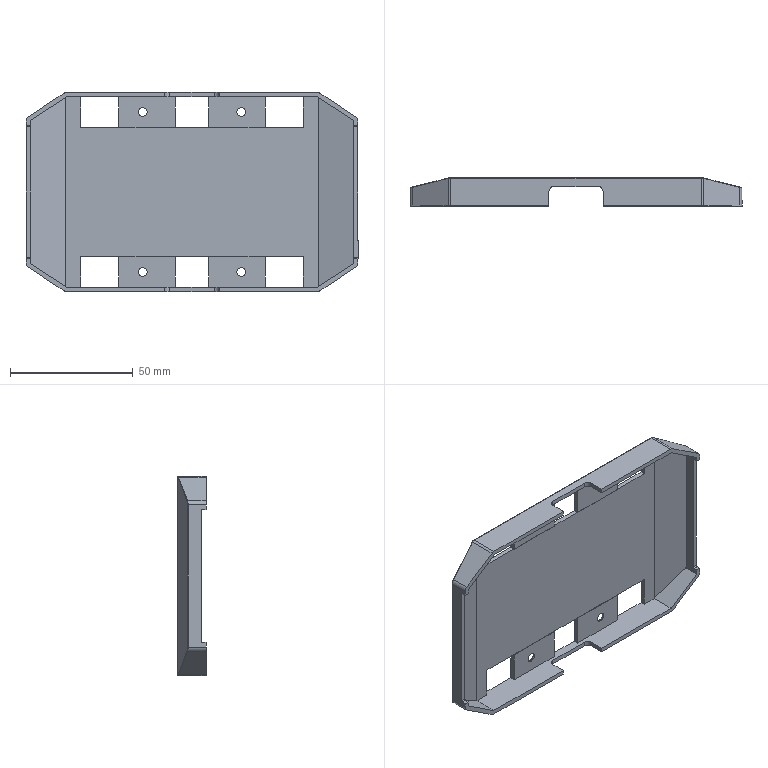Part | NX | features BREP 1 | 1 solid | 126 faces | box 135 x 11.5 x 81 mm | volume 22124 mm3 | plane 64 | cylinder 38 | cone 8 | torus 6 | spline 6 | sphere 4 | commonest cylinder face diameters 0.4 x14 4 x12 3.6 x8 1 x4